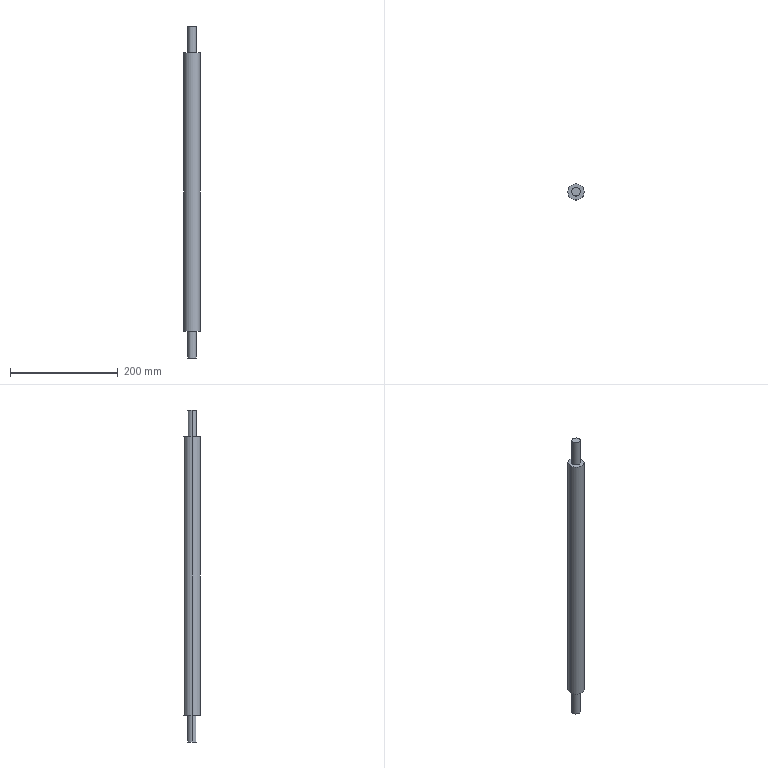Part | SolidWorks | features ICE 2, Extrusion 1 | 1 solid | 10 faces | box 30 x 30 x 615 mm | volume 384138 mm3 | cylinder 6 | plane 4 | commonest cylinder face diameters 16 x4 30 x2
STEP:
#1=CARTESIAN_POINT('',(-8.,0.,-307.5));
#2=VERTEX_POINT('',#1);
#3=CARTESIAN_POINT('',(8.,0.,-307.5));
#4=VERTEX_POINT('',#3);
#5=CARTESIAN_POINT('',(0.,0.,-307.5));
#6=DIRECTION('',(0.,0.,-1.));
#7=DIRECTION('',(-1.,0.,0.));
#8=AXIS2_PLACEMENT_3D('',#5,#6,#7);
#9=CIRCLE('',#8,8.);
#10=EDGE_CURVE('',#2,#4,#9,.T.);
#11=ORIENTED_EDGE('',*,*,#10,.F.);
#12=CARTESIAN_POINT('',(-8.,0.,-257.5));
#13=VERTEX_POINT('',#12);
#14=CARTESIAN_POINT('',(-8.,0.,-307.5));
#15=DIRECTION('',(0.,0.,1.));
#16=VECTOR('',#15,1000.);
#17=LINE('',#14,#16);
#18=EDGE_CURVE('',#2,#13,#17,.T.);
#19=ORIENTED_EDGE('',*,*,#18,.T.);
#20=CARTESIAN_POINT('',(8.,0.,-257.5));
#21=VERTEX_POINT('',#20);
#22=CARTESIAN_POINT('',(0.,0.,-257.5));
#23=DIRECTION('',(0.,0.,-1.));
#24=DIRECTION('',(1.,0.,0.));
#25=AXIS2_PLACEMENT_3D('',#22,#23,#24);
#26=CIRCLE('',#25,8.);
#27=EDGE_CURVE('',#13,#21,#26,.T.);
#28=ORIENTED_EDGE('',*,*,#27,.T.);
#29=CARTESIAN_POINT('',(8.,0.,-307.5));
#30=DIRECTION('',(0.,0.,1.));
#31=VECTOR('',#30,1000.);
#32=LINE('',#29,#31);
#33=EDGE_CURVE('',#4,#21,#32,.T.);
#34=ORIENTED_EDGE('',*,*,#33,.F.);
#35=EDGE_LOOP('',(#11,#19,#28,#34));
#36=FACE_OUTER_BOUND('',#35,.T.);
#37=CARTESIAN_POINT('',(0.,0.,-307.5));
#38=DIRECTION('',(0.,0.,1.));
#39=DIRECTION('',(1.,0.,0.));
#40=AXIS2_PLACEMENT_3D('',#37,#38,#39);
#41=CYLINDRICAL_SURFACE('',#40,8.);
#42=ADVANCED_FACE('',(#36),#41,.T.);
#43=CARTESIAN_POINT('',(8.,0.,307.5));
#44=VERTEX_POINT('',#43);
#45=CARTESIAN_POINT('',(-8.,0.,307.5));
#46=VERTEX_POINT('',#45);
#47=CARTESIAN_POINT('',(0.,0.,307.5));
#48=DIRECTION('',(0.,0.,1.));
#49=DIRECTION('',(1.,0.,0.));
#50=AXIS2_PLACEMENT_3D('',#47,#48,#49);
#51=CIRCLE('',#50,8.);
#52=EDGE_CURVE('',#44,#46,#51,.T.);
#53=ORIENTED_EDGE('',*,*,#52,.F.);
#54=CARTESIAN_POINT('',(8.,0.,257.5));
#55=VERTEX_POINT('',#54);
#56=CARTESIAN_POINT('',(8.,0.,307.5));
#57=DIRECTION('',(0.,0.,-1.));
#58=VECTOR('',#57,1000.);
#59=LINE('',#56,#58);
#60=EDGE_CURVE('',#44,#55,#59,.T.);
#61=ORIENTED_EDGE('',*,*,#60,.T.);
#62=CARTESIAN_POINT('',(-8.,0.,257.5));
#63=VERTEX_POINT('',#62);
#64=CARTESIAN_POINT('',(0.,0.,257.5));
#65=DIRECTION('',(0.,0.,1.));
#66=DIRECTION('',(1.,0.,0.));
#67=AXIS2_PLACEMENT_3D('',#64,#65,#66);
#68=CIRCLE('',#67,8.);
#69=EDGE_CURVE('',#55,#63,#68,.T.);
#70=ORIENTED_EDGE('',*,*,#69,.T.);
#71=CARTESIAN_POINT('',(-8.,0.,307.5));
#72=DIRECTION('',(0.,0.,-1.));
#73=VECTOR('',#72,1000.);
#74=LINE('',#71,#73);
#75=EDGE_CURVE('',#46,#63,#74,.T.);
#76=ORIENTED_EDGE('',*,*,#75,.F.);
#77=EDGE_LOOP('',(#53,#61,#70,#76));
#78=FACE_OUTER_BOUND('',#77,.T.);
#79=CARTESIAN_POINT('',(0.,0.,307.5));
#80=DIRECTION('',(0.,0.,-1.));
#81=DIRECTION('',(-1.,0.,0.));
#82=AXIS2_PLACEMENT_3D('',#79,#80,#81);
#83=CYLINDRICAL_SURFACE('',#82,8.);
#84=ADVANCED_FACE('',(#78),#83,.T.);
#85=CARTESIAN_POINT('',(15.,0.,257.5));
#86=VERTEX_POINT('',#85);
#87=CARTESIAN_POINT('',(-15.,0.,257.5));
#88=VERTEX_POINT('',#87);
#89=CARTESIAN_POINT('',(0.,0.,257.5));
#90=DIRECTION('',(0.,0.,1.));
#91=DIRECTION('',(1.,0.,0.));
#92=AXIS2_PLACEMENT_3D('',#89,#90,#91);
#93=CIRCLE('',#92,15.);
#94=EDGE_CURVE('',#86,#88,#93,.T.);
#95=ORIENTED_EDGE('',*,*,#94,.F.);
#96=CARTESIAN_POINT('',(15.,0.,-257.5));
#97=VERTEX_POINT('',#96);
#98=CARTESIAN_POINT('',(15.,0.,257.5));
#99=DIRECTION('',(0.,0.,-1.));
#100=VECTOR('',#99,1000.);
#101=LINE('',#98,#100);
#102=EDGE_CURVE('',#86,#97,#101,.T.);
#103=ORIENTED_EDGE('',*,*,#102,.T.);
#104=CARTESIAN_POINT('',(-15.,0.,-257.5));
#105=VERTEX_POINT('',#104);
#106=CARTESIAN_POINT('',(0.,0.,-257.5));
#107=DIRECTION('',(0.,0.,1.));
#108=DIRECTION('',(1.,0.,0.));
#109=AXIS2_PLACEMENT_3D('',#106,#107,#108);
#110=CIRCLE('',#109,15.);
#111=EDGE_CURVE('',#97,#105,#110,.T.);
#112=ORIENTED_EDGE('',*,*,#111,.T.);
#113=CARTESIAN_POINT('',(-15.,0.,257.5));
#114=DIRECTION('',(0.,0.,-1.));
#115=VECTOR('',#114,1000.);
#116=LINE('',#113,#115);
#117=EDGE_CURVE('',#88,#105,#116,.T.);
#118=ORIENTED_EDGE('',*,*,#117,.F.);
#119=EDGE_LOOP('',(#95,#103,#112,#118));
#120=FACE_OUTER_BOUND('',#119,.T.);
#121=CARTESIAN_POINT('',(0.,0.,257.5));
#122=DIRECTION('',(0.,0.,-1.));
#123=DIRECTION('',(-1.,0.,0.));
#124=AXIS2_PLACEMENT_3D('',#121,#122,#123);
#125=CYLINDRICAL_SURFACE('',#124,15.);
#126=ADVANCED_FACE('',(#120),#125,.T.);
#127=ORIENTED_EDGE('',*,*,#102,.F.);
#128=CARTESIAN_POINT('',(0.,0.,257.5));
#129=DIRECTION('',(0.,0.,1.));
#130=DIRECTION('',(1.,0.,0.));
#131=AXIS2_PLACEMENT_3D('',#128,#129,#130);
#132=CIRCLE('',#131,15.);
#133=EDGE_CURVE('',#88,#86,#132,.T.);
#134=ORIENTED_EDGE('',*,*,#133,.F.);
#135=ORIENTED_EDGE('',*,*,#117,.T.);
#136=CARTESIAN_POINT('',(0.,0.,-257.5));
#137=DIRECTION('',(0.,0.,1.));
#138=DIRECTION('',(1.,0.,0.));
#139=AXIS2_PLACEMENT_3D('',#136,#137,#138);
#140=CIRCLE('',#139,15.);
#141=EDGE_CURVE('',#105,#97,#140,.T.);
#142=ORIENTED_EDGE('',*,*,#141,.T.);
#143=EDGE_LOOP('',(#127,#134,#135,#142));
#144=FACE_OUTER_BOUND('',#143,.T.);
#145=CARTESIAN_POINT('',(0.,0.,257.5));
#146=DIRECTION('',(0.,0.,-1.));
#147=DIRECTION('',(-1.,0.,0.));
#148=AXIS2_PLACEMENT_3D('',#145,#146,#147);
#149=CYLINDRICAL_SURFACE('',#148,15.);
#150=ADVANCED_FACE('',(#144),#149,.T.);
#151=CARTESIAN_POINT('',(0.,0.,257.5));
#152=DIRECTION('',(0.,0.,1.));
#153=DIRECTION('',(1.,0.,0.));
#154=AXIS2_PLACEMENT_3D('',#151,#152,#153);
#155=CIRCLE('',#154,8.);
#156=EDGE_CURVE('',#63,#55,#155,.T.);
#157=ORIENTED_EDGE('',*,*,#156,.F.);
#158=ORIENTED_EDGE('',*,*,#69,.F.);
#159=EDGE_LOOP('',(#157,#158));
#160=FACE_BOUND('',#159,.T.);
#161=ORIENTED_EDGE('',*,*,#133,.T.);
#162=ORIENTED_EDGE('',*,*,#94,.T.);
#163=EDGE_LOOP('',(#161,#162));
#164=FACE_OUTER_BOUND('',#163,.T.);
#165=CARTESIAN_POINT('',(0.,0.,257.5));
#166=DIRECTION('',(0.,0.,1.));
#167=DIRECTION('',(1.,0.,0.));
#168=AXIS2_PLACEMENT_3D('',#165,#166,#167);
#169=PLANE('',#168);
#170=ADVANCED_FACE('',(#160,#164),#169,.T.);
#171=CARTESIAN_POINT('',(0.,0.,-257.5));
#172=DIRECTION('',(0.,0.,-1.));
#173=DIRECTION('',(1.,0.,0.));
#174=AXIS2_PLACEMENT_3D('',#171,#172,#173);
#175=CIRCLE('',#174,8.);
#176=EDGE_CURVE('',#21,#13,#175,.T.);
#177=ORIENTED_EDGE('',*,*,#176,.F.);
#178=ORIENTED_EDGE('',*,*,#27,.F.);
#179=EDGE_LOOP('',(#177,#178));
#180=FACE_BOUND('',#179,.T.);
#181=ORIENTED_EDGE('',*,*,#141,.F.);
#182=ORIENTED_EDGE('',*,*,#111,.F.);
#183=EDGE_LOOP('',(#181,#182));
#184=FACE_OUTER_BOUND('',#183,.T.);
#185=CARTESIAN_POINT('',(0.,0.,-257.5));
#186=DIRECTION('',(0.,0.,1.));
#187=DIRECTION('',(1.,0.,0.));
#188=AXIS2_PLACEMENT_3D('',#185,#186,#187);
#189=PLANE('',#188);
#190=ADVANCED_FACE('',(#180,#184),#189,.F.);
#191=ORIENTED_EDGE('',*,*,#60,.F.);
#192=CARTESIAN_POINT('',(0.,0.,307.5));
#193=DIRECTION('',(0.,0.,1.));
#194=DIRECTION('',(1.,0.,0.));
#195=AXIS2_PLACEMENT_3D('',#192,#193,#194);
#196=CIRCLE('',#195,8.);
#197=EDGE_CURVE('',#46,#44,#196,.T.);
#198=ORIENTED_EDGE('',*,*,#197,.F.);
#199=ORIENTED_EDGE('',*,*,#75,.T.);
#200=ORIENTED_EDGE('',*,*,#156,.T.);
#201=EDGE_LOOP('',(#191,#198,#199,#200));
#202=FACE_OUTER_BOUND('',#201,.T.);
#203=CARTESIAN_POINT('',(0.,0.,307.5));
#204=DIRECTION('',(0.,0.,-1.));
#205=DIRECTION('',(-1.,0.,0.));
#206=AXIS2_PLACEMENT_3D('',#203,#204,#205);
#207=CYLINDRICAL_SURFACE('',#206,8.);
#208=ADVANCED_FACE('',(#202),#207,.T.);
#209=ORIENTED_EDGE('',*,*,#197,.T.);
#210=ORIENTED_EDGE('',*,*,#52,.T.);
#211=EDGE_LOOP('',(#209,#210));
#212=FACE_OUTER_BOUND('',#211,.T.);
#213=CARTESIAN_POINT('',(0.,0.,307.5));
#214=DIRECTION('',(0.,0.,1.));
#215=DIRECTION('',(1.,0.,0.));
#216=AXIS2_PLACEMENT_3D('',#213,#214,#215);
#217=PLANE('',#216);
#218=ADVANCED_FACE('',(#212),#217,.T.);
#219=ORIENTED_EDGE('',*,*,#18,.F.);
#220=CARTESIAN_POINT('',(0.,0.,-307.5));
#221=DIRECTION('',(0.,0.,-1.));
#222=DIRECTION('',(-1.,0.,0.));
#223=AXIS2_PLACEMENT_3D('',#220,#221,#222);
#224=CIRCLE('',#223,8.);
#225=EDGE_CURVE('',#4,#2,#224,.T.);
#226=ORIENTED_EDGE('',*,*,#225,.F.);
#227=ORIENTED_EDGE('',*,*,#33,.T.);
#228=ORIENTED_EDGE('',*,*,#176,.T.);
#229=EDGE_LOOP('',(#219,#226,#227,#228));
#230=FACE_OUTER_BOUND('',#229,.T.);
#231=CARTESIAN_POINT('',(0.,0.,-307.5));
#232=DIRECTION('',(0.,0.,1.));
#233=DIRECTION('',(1.,0.,0.));
#234=AXIS2_PLACEMENT_3D('',#231,#232,#233);
#235=CYLINDRICAL_SURFACE('',#234,8.);
#236=ADVANCED_FACE('',(#230),#235,.T.);
#237=ORIENTED_EDGE('',*,*,#225,.T.);
#238=ORIENTED_EDGE('',*,*,#10,.T.);
#239=EDGE_LOOP('',(#237,#238));
#240=FACE_OUTER_BOUND('',#239,.T.);
#241=CARTESIAN_POINT('',(0.,0.,-307.5));
#242=DIRECTION('',(0.,0.,-1.));
#243=DIRECTION('',(-1.,0.,0.));
#244=AXIS2_PLACEMENT_3D('',#241,#242,#243);
#245=PLANE('',#244);
#246=ADVANCED_FACE('',(#240),#245,.T.);
#247=CLOSED_SHELL('',(#42,#84,#126,#150,#170,#190,#208,#218,#236,#246));
#248=MANIFOLD_SOLID_BREP('',#247);
#249=CARTESIAN_POINT('',(0.,0.,0.));
#250=DIRECTION('',(0.,0.,1.));
#251=DIRECTION('',(1.,0.,0.));
#252=AXIS2_PLACEMENT_3D('',#249,#250,#251);
#253=(LENGTH_UNIT()NAMED_UNIT(*)SI_UNIT(.MILLI.,.METRE.));
#254=UNCERTAINTY_MEASURE_WITH_UNIT(LENGTH_MEASURE(0.00001),#253,'','');
#255=(NAMED_UNIT(*)PLANE_ANGLE_UNIT()SI_UNIT($,.RADIAN.));
#256=(NAMED_UNIT(*)SI_UNIT($,.STERADIAN.)SOLID_ANGLE_UNIT());
#257=(GEOMETRIC_REPRESENTATION_CONTEXT(3)GLOBAL_UNCERTAINTY_ASSIGNED_CONTEXT((#254))GLOBAL_UNIT_ASSIGNED_CONTEXT((#253,#255,#256))REPRESENTATION_CONTEXT('',''));
#258=ADVANCED_BREP_SHAPE_REPRESENTATION('',(#248,#252),#257);